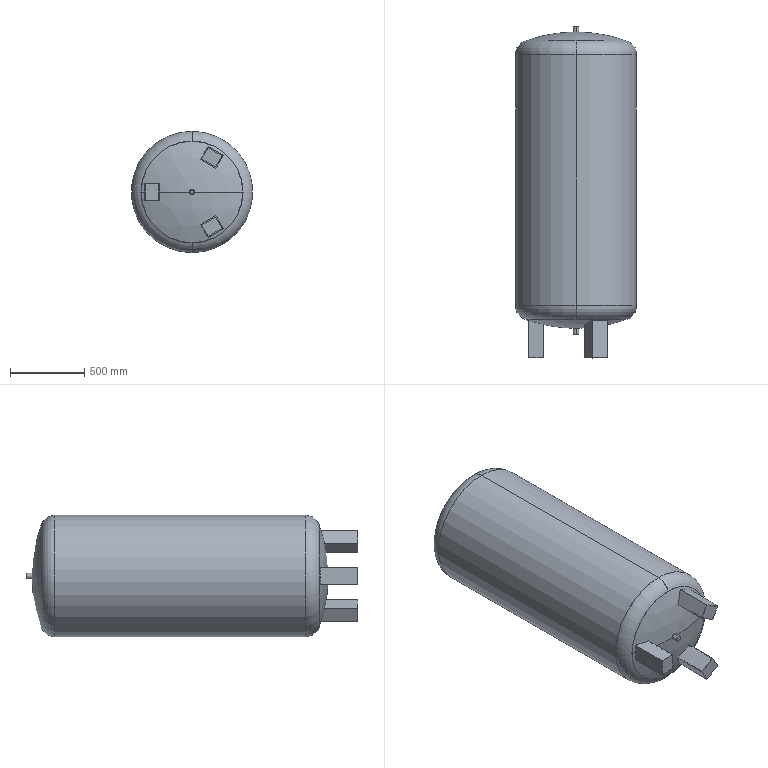Part | SolidWorks | features ICE 2, CirPattern 1, Revolution 1, Shell 1 | 1 solid | 61 faces | box 820 x 2240 x 820 mm | volume 35765153 mm3 | plane 33 | cylinder 12 | torus 8 | sphere 8 | commonest cylinder face diameters 28 x4 40 x4 808 x2 820 x2